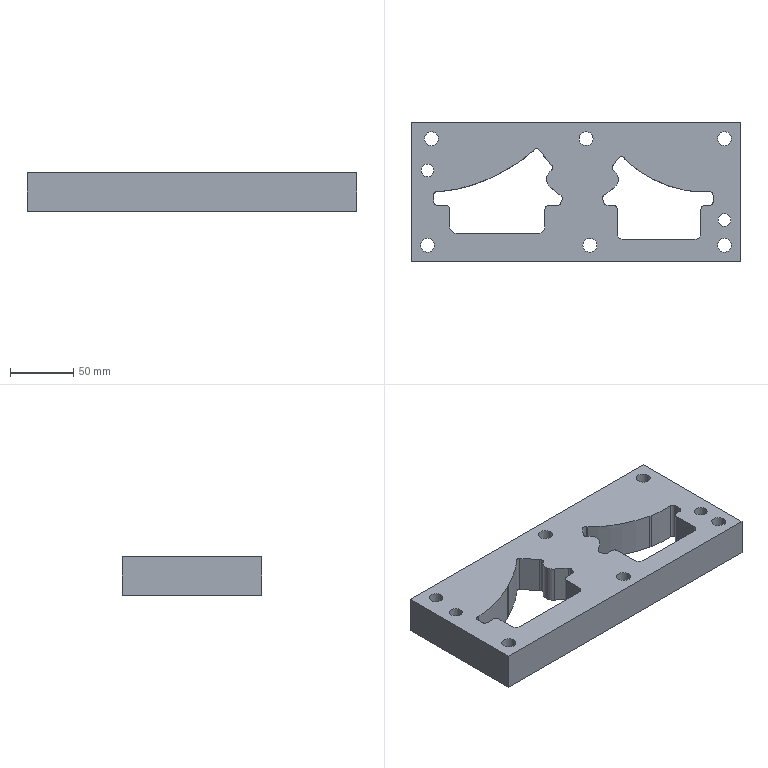Part | STEP file | 203_id734_x_t | 1 solid | 81 faces | box 260 x 110 x 30 mm | volume 603713 mm3 | cylinder 43 | plane 34 | other 4 | commonest cylinder face diameters 5 x13 11 x8 6 x6 10 x6 17 x6 16 x2